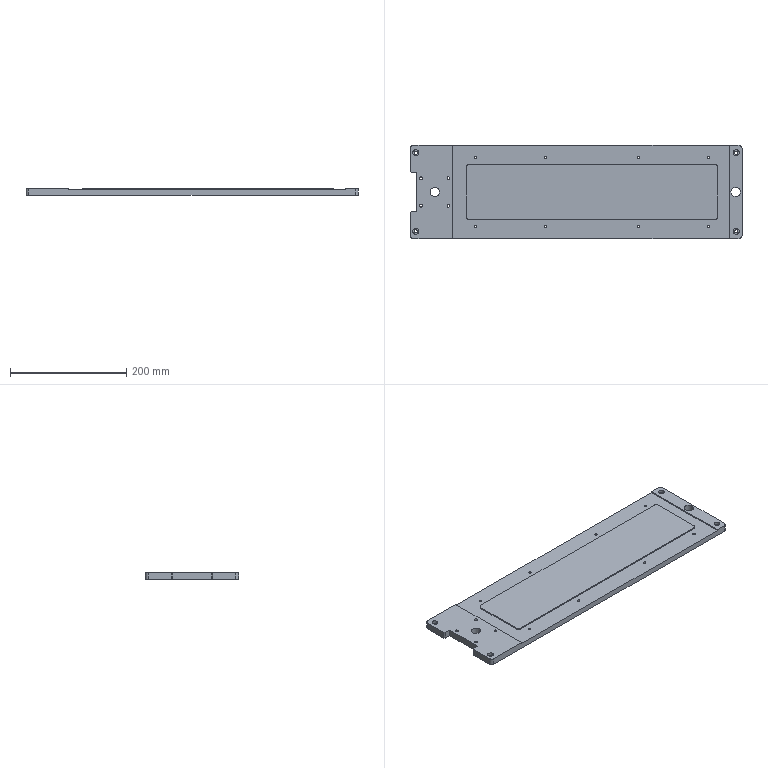Part | SolidWorks | features Cut 3, ICE 3, Fillet 2, HoleWzd 2, Chamfer 1, Extrusion 1 | 1 solid | 77 faces | box 570 x 160 x 12 mm | volume 1005956 mm3 | cylinder 52 | plane 25 | commonest cylinder face diameters 4.2 x16 10 x16 5 x8 5.5 x8 16 x4